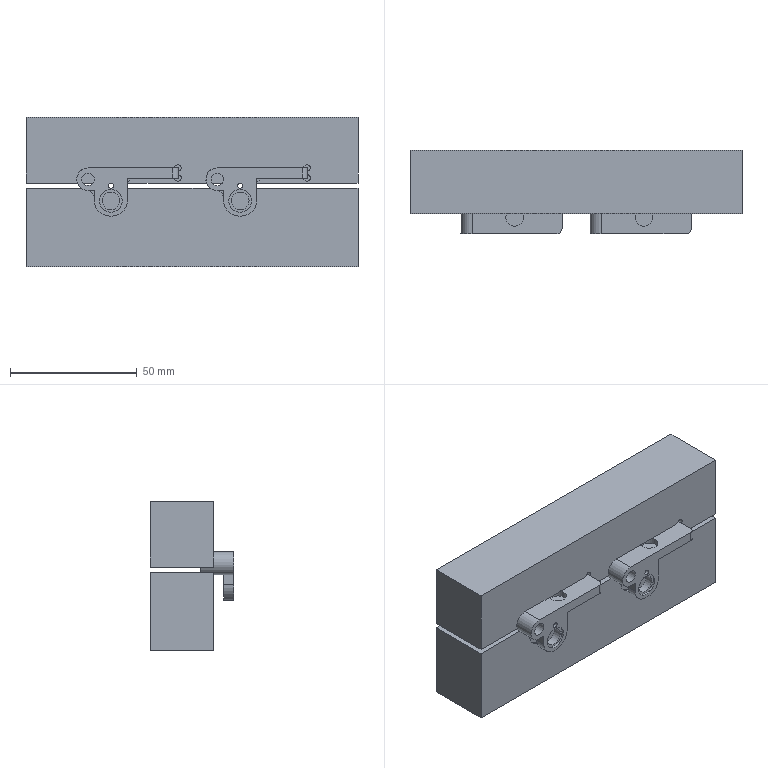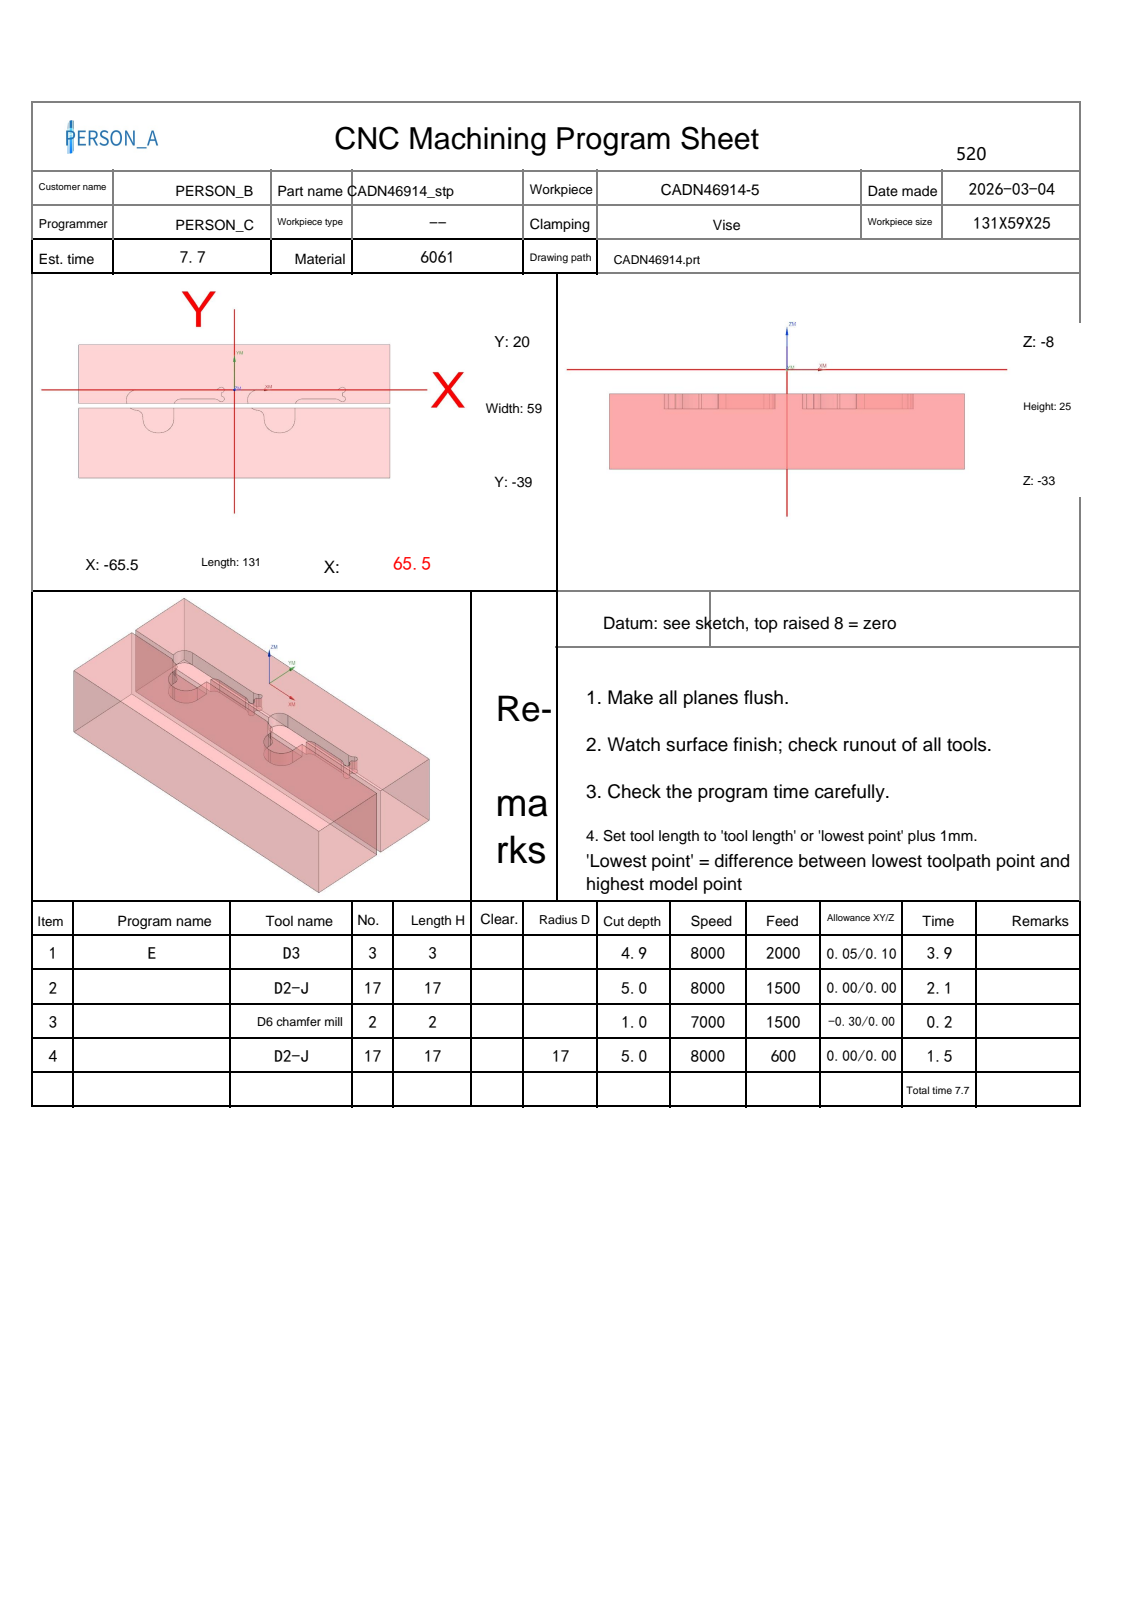NC program | NX | posted by the shop | part box 131 x 33 x 59 mm
Lines 10129 to 10523 of 10523:
N3 T02 M06
(D6 chamfer mill  D=6. R=0. H=02 ce=-0.30 di=0.00)
G00 G90 G54 X-26.819 Y-15.486 M03 S7000
G43 H02 Z40.
M08
Z-5.5
G01 X-26.635 Y-15.111 Z-5.652 F1500.
X-26.459 Y-14.646 Z-5.833
X-26.327 Y-14.165 Z-6.015
X-26.24 Y-13.675 Z-6.196
X-26.2 Y-13.178 Z-6.377
Y-7.97 Z-8.273
X-26.029 Y-5.979 Z-9.
G02 X-25.971 Y-5.719 I.996 J-.085
X-22.5 Y-3.3 I3.471 J-1.281
G01 X-8.51
G02 X-5.89 Y-4.388 I0.0 J-3.7
G03 X-5.5 Y-4.55 I.39 J.388
X-4.95 Y-4. I0.0 J.55
X-5.394 Y-3.46 I-.55 J0.0
G02 X-6.2 Y-2.479 I.194 J.981
G01 Y-1.521
G02 X-5.394 Y-.54 I1. J0.0
G03 X-4.95 Y0.0 I-.106 J.54
X-5.5 Y.55 I-.55 J0.0
X-5.89 Y.388 I0.0 J-.55
G02 X-8.51 Y-.7 I-2.621 J2.612
G01 X-41.
G03 X-44.8 Y-4.5 I0.0 J-3.8
X-41.253 Y-8.292 I3.8 J0.0
G02 X-37.8 Y-11.983 I-.247 J-3.692
G01 Y-13.
G03 X-32.5 Y-18.3 I5.3 J0.0
G01 X-31.5
G03 X-26.2 Y-13. I0.0 J5.3
G01 Y-8.013
X-26.202 Y-7.97
X-26.196 Y-7.927
X-26.029 Y-5.979
G02 X-25.971 Y-5.719 I.996 J-.085
X-25.884 Y-5.504 I3.471 J-1.281
G01 Z-6.5
G00 Z40.
X24.181 Y-15.486
Z-5.5
G01 X24.365 Y-15.111 Z-5.652
X24.541 Y-14.646 Z-5.833
X24.673 Y-14.165 Z-6.015
X24.76 Y-13.675 Z-6.196
X24.8 Y-13.178 Z-6.377
Y-7.97 Z-8.273
X24.971 Y-5.979 Z-9.
G02 X25.029 Y-5.719 I.996 J-.085
X28.5 Y-3.3 I3.471 J-1.281
G01 X42.49
G02 X45.11 Y-4.388 I0.0 J-3.7
G03 X45.5 Y-4.55 I.39 J.388
X46.05 Y-4. I0.0 J.55
X45.606 Y-3.46 I-.55 J0.0
G02 X44.8 Y-2.479 I.194 J.981
G01 Y-1.521
G02 X45.606 Y-.54 I1. J0.0
G03 X46.05 Y0.0 I-.106 J.54
X45.5 Y.55 I-.55 J0.0
X45.11 Y.388 I0.0 J-.55
G02 X42.49 Y-.7 I-2.621 J2.612
G01 X10.
G03 X6.2 Y-4.5 I0.0 J-3.8
X9.747 Y-8.292 I3.8 J0.0
G02 X13.2 Y-11.983 I-.247 J-3.692
G01 Y-13.
G03 X18.5 Y-18.3 I5.3 J0.0
G01 X19.5
G03 X24.8 Y-13. I0.0 J5.3
G01 Y-8.013
X24.798 Y-7.97
X24.804 Y-7.927
X24.971 Y-5.979
G02 X25.029 Y-5.719 I.996 J-.085
X25.116 Y-5.504 I3.471 J-1.281
G01 Z-6.5
G00 Z40.
G91 G28 Z0.0
M05
M09
G91 G28 Z0.0
M01
N4 T17 M06
(D2-J  D=2. R=0. H=17 ce=0.00 di=0.00)
G00 G90 G54 X-43.492 Y-6.523 M03 S8000
G43 H17 Z2.
M08
Z-9.
G01 Z-10.5 F600.
G41 D17
X-43.69 Y-6.492
X-43.737 Y-6.489
G03 X-43.97 Y-6.6 I0.0 J-.3
G01 X-43.2 Y-7.222
G03 X-41.233 Y-7.992 I2.2 J2.722
G02 X-37.5 Y-11.983 I-.267 J-3.991
G01 Y-13.
G03 X-32.5 Y-18. I5. J0.0
G01 X-31.5
G03 X-26.5 Y-13. I0.0 J5.
G01 Y-7.
G03 X-26.8 Y-7.3 I0.0 J-.3
G01 G40 Y-7.5
Z-9.
G00 X-43.492 Y-6.523
Z-11.5
G01 Z-13.
G41 D17
X-43.69 Y-6.492
X-43.737 Y-6.489
G03 X-43.97 Y-6.6 I0.0 J-.3
G01 X-43.2 Y-7.222
G03 X-41.233 Y-7.992 I2.2 J2.722
G02 X-37.5 Y-11.983 I-.267 J-3.991
G01 Y-13.
G03 X-32.5 Y-18. I5. J0.0
G01 X-31.5
G03 X-26.5 Y-13. I0.0 J5.
G01 Y-7.
G03 X-26.8 Y-6.7 I-.3 J0.0
G01 X-26.955
G40 X-27.155
Z-11.5
G00 Z2.
X7.508 Y-6.523
Z-9.
G01 Z-10.5
G41 D17
X7.31 Y-6.492
X7.263 Y-6.489
G03 X7.03 Y-6.6 I0.0 J-.3
G01 X7.8 Y-7.222
G03 X9.767 Y-7.992 I2.2 J2.722
G02 X13.5 Y-11.983 I-.267 J-3.991
G01 Y-13.
G03 X18.5 Y-18. I5. J0.0
G01 X19.5
G03 X24.5 Y-13. I0.0 J5.
G01 Y-7.
G03 X24.2 Y-7.3 I0.0 J-.3
G01 G40 Y-7.5
Z-9.
G00 X7.508 Y-6.523
Z-11.5
G01 Z-13.
G41 D17
X7.31 Y-6.492
X7.263 Y-6.489
G03 X7.03 Y-6.6 I0.0 J-.3
G01 X7.8 Y-7.222
G03 X9.767 Y-7.992 I2.2 J2.722
G02 X13.5 Y-11.983 I-.267 J-3.991
G01 Y-13.
G03 X18.5 Y-18. I5. J0.0
G01 X19.5
G03 X24.5 Y-13. I0.0 J5.
G01 Y-7.
G03 X24.2 Y-7.3 I0.0 J-.3
G01 G40 Y-7.5
Z-11.5
G00 Z2.
G00 G90 X23.824 Y-6.726 M03 S8000
Z2.
Z-7.5
G01 Z-9. F600.
G41 D17
X24.013 Y-6.792
X24.113 Y-6.809
G03 X24.395 Y-6.609 I0.0 J.3
G01 X24.729 Y-5.667
G02 X28.5 Y-3. I3.771 J-1.333
G01 X42.49
G02 X44.5 Y-3.542 I0.0 J-4.
G01 Y-.458
G02 X42.49 Y-1. I-2.01 J3.458
G01 X10.
G03 X6.5 Y-4.5 I0.0 J-3.5
X6.7 Y-5.667 I3.5 J0.0
G01 X7.034 Y-6.609
G03 X7.316 Y-6.809 I.283 J.1
G01 X7.416 Y-6.792
X7.645 Y-6.711
G40 X7.834 Y-6.645
Z-7.5
G00 X23.824 Y-6.726
Z-8.5
G01 Z-10.
G41 D17
X24.013 Y-6.792
X24.113 Y-6.809
G03 X24.395 Y-6.609 I0.0 J.3
G01 X24.729 Y-5.667
G02 X28.5 Y-3. I3.771 J-1.333
G01 X42.49
G02 X44.5 Y-3.542 I0.0 J-4.
G01 Y-.458
G02 X42.49 Y-1. I-2.01 J3.458
G01 X10.
G03 X6.5 Y-4.5 I0.0 J-3.5
X6.7 Y-5.667 I3.5 J0.0
G01 X7.034 Y-6.609
G03 X7.316 Y-6.809 I.283 J.1
G01 X7.416 Y-6.792
X7.645 Y-6.711
G40 X7.834 Y-6.645
Z-8.5
G00 X23.824 Y-6.726
Z-9.5
G01 Z-11.
G41 D17
X24.013 Y-6.792
X24.113 Y-6.809
G03 X24.395 Y-6.609 I0.0 J.3
G01 X24.729 Y-5.667
G02 X28.5 Y-3. I3.771 J-1.333
G01 X42.49
G02 X44.5 Y-3.542 I0.0 J-4.
G01 Y-.458
G02 X42.49 Y-1. I-2.01 J3.458
G01 X10.
G03 X6.5 Y-4.5 I0.0 J-3.5
X6.7 Y-5.667 I3.5 J0.0
G01 X7.034 Y-6.609
G03 X7.316 Y-6.809 I.283 J.1
G01 X7.416 Y-6.792
X7.645 Y-6.711
G40 X7.834 Y-6.645
Z-9.5
G00 X23.823 Y-6.728
Z-10.5
G01 Z-12.
G41 D17
X24.012 Y-6.795
X24.112 Y-6.812
G03 X24.394 Y-6.612 I0.0 J.3
G01 X24.729 Y-5.667
G02 X28.5 Y-3. I3.771 J-1.333
G01 X42.49
G02 X44.5 Y-3.542 I0.0 J-4.
G01 Y-.458
G02 X42.49 Y-1. I-2.01 J3.458
G01 X10.
G03 X6.5 Y-4.5 I0.0 J-3.5
X6.7 Y-5.667 I3.5 J0.0
G01 X7.034 Y-6.609
G03 X7.316 Y-6.809 I.283 J.1
G01 X7.416 Y-6.792
X7.645 Y-6.711
G40 X7.834 Y-6.645
Z-10.5
G00 X23.823 Y-6.728
Z-11.5
G01 Z-13.
G41 D17
X24.012 Y-6.795
X24.112 Y-6.812
G03 X24.394 Y-6.612 I0.0 J.3
G01 X24.729 Y-5.667
G02 X28.5 Y-3. I3.771 J-1.333
G01 X42.49
G02 X44.5 Y-3.542 I0.0 J-4.
G01 Y-.458
G02 X42.49 Y-1. I-2.01 J3.458
G01 X10.
G03 X6.5 Y-4.5 I0.0 J-3.5
X6.7 Y-5.667 I3.5 J0.0
G01 X7.034 Y-6.609
G03 X7.316 Y-6.809 I.283 J.1
G01 X7.416 Y-6.792
X7.645 Y-6.711
G40 X7.834 Y-6.645
Z-11.5
G00 Z2.
X-27.176 Y-6.726
Z-7.5
G01 Z-9.
G41 D17
X-26.987 Y-6.792
X-26.887 Y-6.809
G03 X-26.605 Y-6.609 I0.0 J.3
G01 X-26.271 Y-5.667
G02 X-22.5 Y-3. I3.771 J-1.333
G01 X-8.51
G02 X-6.5 Y-3.542 I0.0 J-4.
G01 Y-.458
G02 X-8.51 Y-1. I-2.01 J3.458
G01 X-41.
G03 X-44.5 Y-4.5 I0.0 J-3.5
X-44.3 Y-5.667 I3.5 J0.0
G01 X-43.966 Y-6.609
G03 X-43.684 Y-6.809 I.283 J.1
G01 X-43.584 Y-6.792
X-43.355 Y-6.711
G40 X-43.166 Y-6.645
Z-7.5
G00 X-27.176 Y-6.726
Z-8.5
G01 Z-10.
G41 D17
X-26.987 Y-6.792
X-26.887 Y-6.809
G03 X-26.605 Y-6.609 I0.0 J.3
G01 X-26.271 Y-5.667
G02 X-22.5 Y-3. I3.771 J-1.333
G01 X-8.51
G02 X-6.5 Y-3.542 I0.0 J-4.
G01 Y-.458
G02 X-8.51 Y-1. I-2.01 J3.458
G01 X-41.
G03 X-44.5 Y-4.5 I0.0 J-3.5
X-44.3 Y-5.667 I3.5 J0.0
G01 X-43.966 Y-6.609
G03 X-43.684 Y-6.809 I.283 J.1
G01 X-43.584 Y-6.792
X-43.355 Y-6.711
G40 X-43.166 Y-6.645
Z-8.5
G00 X-27.176 Y-6.726
Z-9.5
G01 Z-11.
G41 D17
X-26.987 Y-6.792
X-26.887 Y-6.809
G03 X-26.605 Y-6.609 I0.0 J.3
G01 X-26.271 Y-5.667
G02 X-22.5 Y-3. I3.771 J-1.333
G01 X-8.51
G02 X-6.5 Y-3.542 I0.0 J-4.
G01 Y-.458
G02 X-8.51 Y-1. I-2.01 J3.458
G01 X-41.
G03 X-44.5 Y-4.5 I0.0 J-3.5
X-44.3 Y-5.667 I3.5 J0.0
G01 X-43.966 Y-6.609
G03 X-43.684 Y-6.809 I.283 J.1
G01 X-43.584 Y-6.792
X-43.355 Y-6.711
G40 X-43.166 Y-6.645
Z-9.5
G00 X-27.176 Y-6.726
Z-10.5
G01 Z-12.
G41 D17
X-26.987 Y-6.792
X-26.887 Y-6.809
G03 X-26.605 Y-6.609 I0.0 J.3
G01 X-26.271 Y-5.667
G02 X-22.5 Y-3. I3.771 J-1.333
G01 X-8.51
G02 X-6.5 Y-3.542 I0.0 J-4.
G01 Y-.458
G02 X-8.51 Y-1. I-2.01 J3.458
G01 X-41.
G03 X-44.5 Y-4.5 I0.0 J-3.5
X-44.3 Y-5.667 I3.5 J0.0
G01 X-43.966 Y-6.612
G03 X-43.683 Y-6.812 I.283 J.1
G01 X-43.583 Y-6.795
X-43.352 Y-6.714
G40 X-43.163 Y-6.647
Z-10.5
G00 X-27.176 Y-6.726
Z-11.5
G01 Z-13.
G41 D17
X-26.987 Y-6.792
X-26.887 Y-6.809
G03 X-26.605 Y-6.609 I0.0 J.3
G01 X-26.271 Y-5.667
G02 X-22.5 Y-3. I3.771 J-1.333
G01 X-8.51
G02 X-6.5 Y-3.542 I0.0 J-4.
G01 Y-.458
G02 X-8.51 Y-1. I-2.01 J3.458
G01 X-41.
G03 X-44.5 Y-4.5 I0.0 J-3.5
X-44.3 Y-5.667 I3.5 J0.0
G01 X-43.966 Y-6.612
G03 X-43.683 Y-6.812 I.283 J.1
G01 X-43.583 Y-6.795
X-43.352 Y-6.714
G40 X-43.163 Y-6.647
Z-11.5
G00 Z2.
M05
M09
G91 G28 Z0.0
G91 G28 Y0.0
M30
%